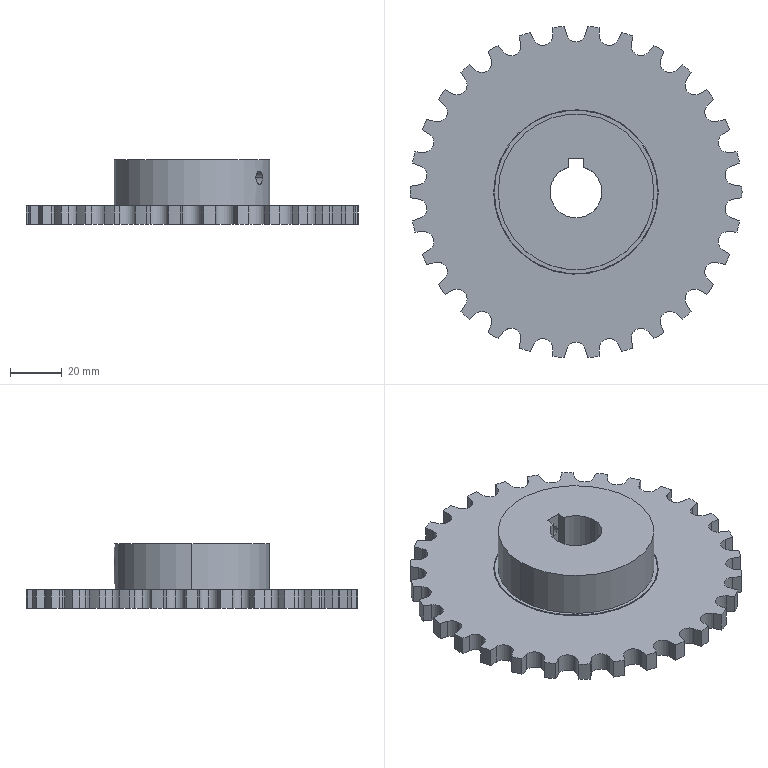Part | STEP file | 1004-2001-0089_1004-2001-0089_1-2 | 1 solid | 153 faces | box 128 x 127.688 x 25 mm | volume 124903 mm3 | cylinder 84 | plane 67 | spline 2 | commonest cylinder face diameters 7.5 x42 128 x31 5 x4 20 x3 60 x2 63 x2